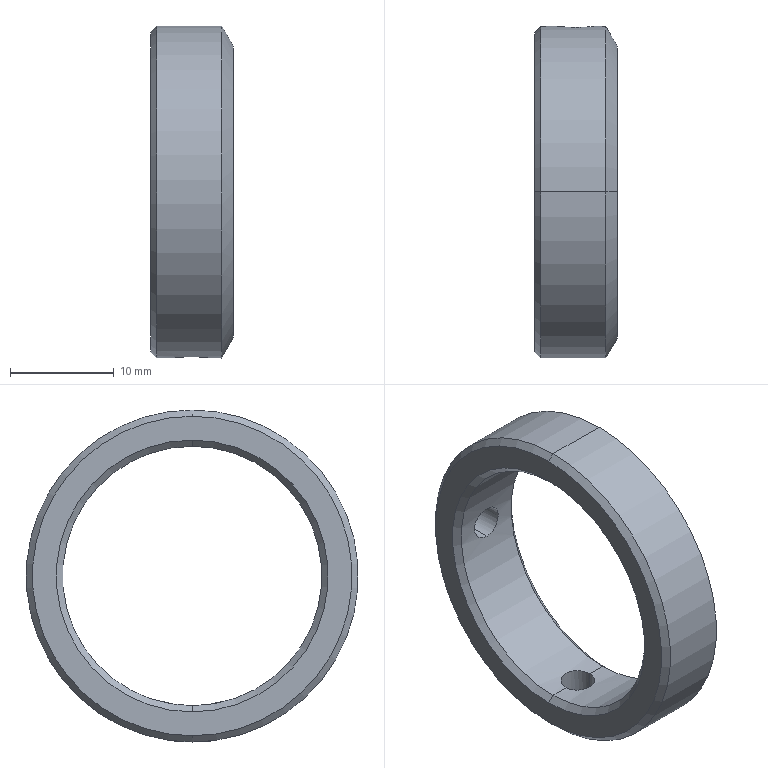Part | STEP file | 1 solid | 22 faces | box 8 x 32 x 32 mm | volume 2296 mm3 | cone 12 | cylinder 8 | plane 2 | commonest cylinder face diameters 3.242 x4 25 x2 32 x2